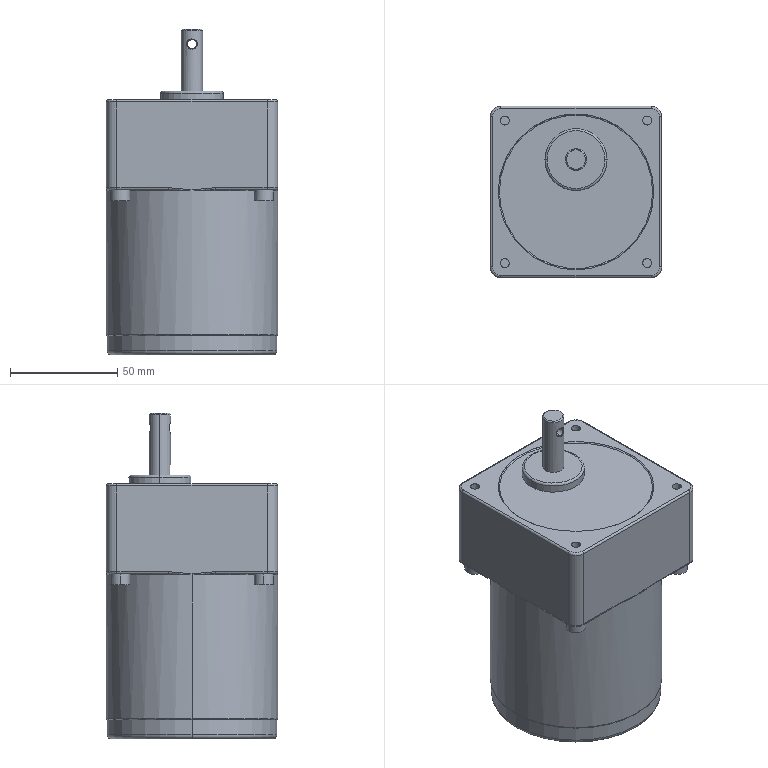Part | STEP file | 102000010056 | 1 solid | 163 faces | box 80 x 80 x 152 mm | volume 651211 mm3 | plane 51 | cylinder 46 | spline 40 | torus 24 | cone 2 | commonest cylinder face diameters 2 x12 4.2 x8 9 x8 10 x6 4.1 x2 29 x2